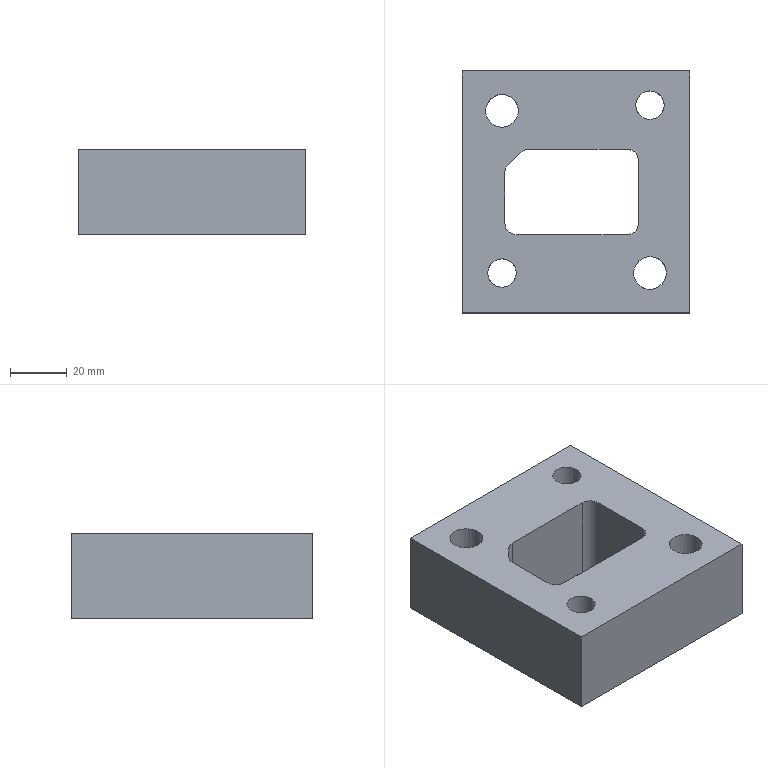Part | NX | features 7 2 | 1 solid | 28 faces | box 80 x 85 x 30 mm | volume 147731 mm3 | plane 15 | cylinder 13 | commonest cylinder face diameters 8 x5 10.001 x2 10.31 x2 11.5 x2 18 x2
STEP:
#1=CARTESIAN_POINT('',(3138.247,112.829,91.));
#2=VERTEX_POINT('',#1);
#3=CARTESIAN_POINT('',(3138.247,107.828,91.));
#4=DIRECTION('',(0.,0.,-1.));
#5=DIRECTION('',(0.,1.,0.));
#6=AXIS2_PLACEMENT_3D('',#3,#4,#5);
#7=CIRCLE('',#6,5.);
#8=EDGE_CURVE('',#2,#2,#7,.T.);
#9=ORIENTED_EDGE('',*,*,#8,.T.);
#10=EDGE_LOOP('',(#9));
#11=FACE_BOUND('',#10,.T.);
#12=CARTESIAN_POINT('',(3086.247,111.578,91.));
#13=VERTEX_POINT('',#12);
#14=CARTESIAN_POINT('',(3086.247,105.828,91.));
#15=DIRECTION('',(0.,0.,1.));
#16=DIRECTION('',(0.,1.,0.));
#17=AXIS2_PLACEMENT_3D('',#14,#15,#16);
#18=CIRCLE('',#17,5.75);
#19=EDGE_CURVE('',#13,#13,#18,.T.);
#20=ORIENTED_EDGE('',*,*,#19,.F.);
#21=EDGE_LOOP('',(#20));
#22=FACE_BOUND('',#21,.T.);
#23=CARTESIAN_POINT('',(3152.247,34.828,91.));
#24=VERTEX_POINT('',#23);
#25=CARTESIAN_POINT('',(3072.247,34.828,91.));
#26=VERTEX_POINT('',#25);
#27=CARTESIAN_POINT('',(3102.247,34.828,91.));
#28=DIRECTION('',(-1.,0.,0.));
#29=VECTOR('',#28,1000.);
#30=LINE('',#27,#29);
#31=EDGE_CURVE('',#24,#26,#30,.T.);
#32=ORIENTED_EDGE('',*,*,#31,.F.);
#33=CARTESIAN_POINT('',(3152.247,119.828,91.));
#34=VERTEX_POINT('',#33);
#35=CARTESIAN_POINT('',(3152.247,77.328,91.));
#36=DIRECTION('',(0.,-1.,0.));
#37=VECTOR('',#36,1000.);
#38=LINE('',#35,#37);
#39=EDGE_CURVE('',#34,#24,#38,.T.);
#40=ORIENTED_EDGE('',*,*,#39,.F.);
#41=CARTESIAN_POINT('',(3072.247,119.828,91.));
#42=VERTEX_POINT('',#41);
#43=CARTESIAN_POINT('',(3102.247,119.828,91.));
#44=DIRECTION('',(1.,0.,0.));
#45=VECTOR('',#44,1000.);
#46=LINE('',#43,#45);
#47=EDGE_CURVE('',#42,#34,#46,.T.);
#48=ORIENTED_EDGE('',*,*,#47,.F.);
#49=CARTESIAN_POINT('',(3072.247,77.328,91.));
#50=DIRECTION('',(0.,1.,0.));
#51=VECTOR('',#50,1000.);
#52=LINE('',#49,#51);
#53=EDGE_CURVE('',#26,#42,#52,.T.);
#54=ORIENTED_EDGE('',*,*,#53,.F.);
#55=EDGE_LOOP('',(#32,#40,#48,#54));
#56=FACE_BOUND('',#55,.T.);
#57=CARTESIAN_POINT('',(3138.247,54.578,91.));
#58=VERTEX_POINT('',#57);
#59=CARTESIAN_POINT('',(3138.247,48.828,91.));
#60=DIRECTION('',(0.,0.,1.));
#61=DIRECTION('',(0.,1.,0.));
#62=AXIS2_PLACEMENT_3D('',#59,#60,#61);
#63=CIRCLE('',#62,5.75);
#64=EDGE_CURVE('',#58,#58,#63,.T.);
#65=ORIENTED_EDGE('',*,*,#64,.F.);
#66=EDGE_LOOP('',(#65));
#67=FACE_BOUND('',#66,.T.);
#68=CARTESIAN_POINT('',(3086.247,53.829,91.));
#69=VERTEX_POINT('',#68);
#70=CARTESIAN_POINT('',(3086.247,48.828,91.));
#71=DIRECTION('',(0.,0.,-1.));
#72=DIRECTION('',(0.,1.,0.));
#73=AXIS2_PLACEMENT_3D('',#70,#71,#72);
#74=CIRCLE('',#73,5.);
#75=EDGE_CURVE('',#69,#69,#74,.T.);
#76=ORIENTED_EDGE('',*,*,#75,.T.);
#77=EDGE_LOOP('',(#76));
#78=FACE_BOUND('',#77,.T.);
#79=CARTESIAN_POINT('',(3130.247,62.328,91.));
#80=VERTEX_POINT('',#79);
#81=CARTESIAN_POINT('',(3134.247,66.328,91.));
#82=VERTEX_POINT('',#81);
#83=CARTESIAN_POINT('',(3130.247,66.328,91.));
#84=DIRECTION('',(0.,0.,1.));
#85=DIRECTION('',(0.,1.,0.));
#86=AXIS2_PLACEMENT_3D('',#83,#84,#85);
#87=CIRCLE('',#86,4.);
#88=EDGE_CURVE('',#80,#82,#87,.T.);
#89=ORIENTED_EDGE('',*,*,#88,.F.);
#90=CARTESIAN_POINT('',(3091.247,62.328,91.));
#91=VERTEX_POINT('',#90);
#92=CARTESIAN_POINT('',(3102.247,62.328,91.));
#93=DIRECTION('',(-1.,0.,0.));
#94=VECTOR('',#93,1000.);
#95=LINE('',#92,#94);
#96=EDGE_CURVE('',#80,#91,#95,.T.);
#97=ORIENTED_EDGE('',*,*,#96,.T.);
#98=CARTESIAN_POINT('',(3087.247,66.328,91.));
#99=VERTEX_POINT('',#98);
#100=CARTESIAN_POINT('',(3091.247,66.328,91.));
#101=DIRECTION('',(0.,0.,1.));
#102=DIRECTION('',(0.,1.,0.));
#103=AXIS2_PLACEMENT_3D('',#100,#101,#102);
#104=CIRCLE('',#103,4.);
#105=EDGE_CURVE('',#99,#91,#104,.T.);
#106=ORIENTED_EDGE('',*,*,#105,.F.);
#107=CARTESIAN_POINT('',(3087.247,84.035,91.));
#108=VERTEX_POINT('',#107);
#109=CARTESIAN_POINT('',(3087.247,77.328,91.));
#110=DIRECTION('',(0.,1.,0.));
#111=VECTOR('',#110,1000.);
#112=LINE('',#109,#111);
#113=EDGE_CURVE('',#99,#108,#112,.T.);
#114=ORIENTED_EDGE('',*,*,#113,.T.);
#115=CARTESIAN_POINT('',(3088.419,86.864,91.));
#116=VERTEX_POINT('',#115);
#117=CARTESIAN_POINT('',(3091.247,84.035,91.));
#118=DIRECTION('',(0.,0.,1.));
#119=DIRECTION('',(0.,1.,0.));
#120=AXIS2_PLACEMENT_3D('',#117,#118,#119);
#121=CIRCLE('',#120,4.);
#122=EDGE_CURVE('',#116,#108,#121,.T.);
#123=ORIENTED_EDGE('',*,*,#122,.F.);
#124=CARTESIAN_POINT('',(3092.711,91.157,91.));
#125=VERTEX_POINT('',#124);
#126=CARTESIAN_POINT('',(3091.815,90.26,91.));
#127=DIRECTION('',(-0.7071,-0.7071,0.));
#128=VECTOR('',#127,1000.);
#129=LINE('',#126,#128);
#130=EDGE_CURVE('',#125,#116,#129,.T.);
#131=ORIENTED_EDGE('',*,*,#130,.F.);
#132=CARTESIAN_POINT('',(3095.54,92.328,91.));
#133=VERTEX_POINT('',#132);
#134=CARTESIAN_POINT('',(3095.54,88.328,91.));
#135=DIRECTION('',(0.,0.,1.));
#136=DIRECTION('',(0.,1.,0.));
#137=AXIS2_PLACEMENT_3D('',#134,#135,#136);
#138=CIRCLE('',#137,4.);
#139=EDGE_CURVE('',#133,#125,#138,.T.);
#140=ORIENTED_EDGE('',*,*,#139,.F.);
#141=CARTESIAN_POINT('',(3130.247,92.328,91.));
#142=VERTEX_POINT('',#141);
#143=CARTESIAN_POINT('',(3102.247,92.328,91.));
#144=DIRECTION('',(1.,0.,0.));
#145=VECTOR('',#144,1000.);
#146=LINE('',#143,#145);
#147=EDGE_CURVE('',#133,#142,#146,.T.);
#148=ORIENTED_EDGE('',*,*,#147,.T.);
#149=CARTESIAN_POINT('',(3134.247,88.328,91.));
#150=VERTEX_POINT('',#149);
#151=CARTESIAN_POINT('',(3130.247,88.328,91.));
#152=DIRECTION('',(0.,0.,1.));
#153=DIRECTION('',(0.,1.,0.));
#154=AXIS2_PLACEMENT_3D('',#151,#152,#153);
#155=CIRCLE('',#154,4.);
#156=EDGE_CURVE('',#150,#142,#155,.T.);
#157=ORIENTED_EDGE('',*,*,#156,.F.);
#158=CARTESIAN_POINT('',(3134.247,77.328,91.));
#159=DIRECTION('',(0.,-1.,0.));
#160=VECTOR('',#159,1000.);
#161=LINE('',#158,#160);
#162=EDGE_CURVE('',#150,#82,#161,.T.);
#163=ORIENTED_EDGE('',*,*,#162,.T.);
#164=EDGE_LOOP('',(#89,#97,#106,#114,#123,#131,#140,#148,#157,#163));
#165=FACE_BOUND('',#164,.T.);
#166=CARTESIAN_POINT('',(3102.247,77.328,91.));
#167=DIRECTION('',(0.,0.,1.));
#168=DIRECTION('',(0.,-1.,0.));
#169=AXIS2_PLACEMENT_3D('',#166,#167,#168);
#170=PLANE('',#169);
#171=ADVANCED_FACE('',(#11,#22,#56,#67,#78,#165),#170,.T.);
#172=CARTESIAN_POINT('',(3143.402,107.828,61.));
#173=VERTEX_POINT('',#172);
#174=CARTESIAN_POINT('',(3138.247,107.828,61.));
#175=DIRECTION('',(0.,0.,1.));
#176=DIRECTION('',(1.,0.,0.));
#177=AXIS2_PLACEMENT_3D('',#174,#175,#176);
#178=CIRCLE('',#177,5.155);
#179=EDGE_CURVE('',#173,#173,#178,.T.);
#180=ORIENTED_EDGE('',*,*,#179,.T.);
#181=EDGE_LOOP('',(#180));
#182=FACE_BOUND('',#181,.T.);
#183=CARTESIAN_POINT('',(3091.402,48.828,61.));
#184=VERTEX_POINT('',#183);
#185=CARTESIAN_POINT('',(3086.247,48.828,61.));
#186=DIRECTION('',(0.,0.,1.));
#187=DIRECTION('',(1.,0.,0.));
#188=AXIS2_PLACEMENT_3D('',#185,#186,#187);
#189=CIRCLE('',#188,5.155);
#190=EDGE_CURVE('',#184,#184,#189,.T.);
#191=ORIENTED_EDGE('',*,*,#190,.T.);
#192=EDGE_LOOP('',(#191));
#193=FACE_BOUND('',#192,.T.);
#194=CARTESIAN_POINT('',(3072.247,119.828,61.));
#195=VERTEX_POINT('',#194);
#196=CARTESIAN_POINT('',(3072.247,34.828,61.));
#197=VERTEX_POINT('',#196);
#198=CARTESIAN_POINT('',(3072.247,-99.672,61.));
#199=DIRECTION('',(0.,-1.,0.));
#200=VECTOR('',#199,1000.);
#201=LINE('',#198,#200);
#202=EDGE_CURVE('',#195,#197,#201,.T.);
#203=ORIENTED_EDGE('',*,*,#202,.F.);
#204=CARTESIAN_POINT('',(3152.247,119.828,61.));
#205=VERTEX_POINT('',#204);
#206=CARTESIAN_POINT('',(3287.247,119.828,61.));
#207=DIRECTION('',(-1.,0.,0.));
#208=VECTOR('',#207,1000.);
#209=LINE('',#206,#208);
#210=EDGE_CURVE('',#205,#195,#209,.T.);
#211=ORIENTED_EDGE('',*,*,#210,.F.);
#212=CARTESIAN_POINT('',(3152.247,34.828,61.));
#213=VERTEX_POINT('',#212);
#214=CARTESIAN_POINT('',(3152.247,-99.672,61.));
#215=DIRECTION('',(0.,1.,0.));
#216=VECTOR('',#215,1000.);
#217=LINE('',#214,#216);
#218=EDGE_CURVE('',#213,#205,#217,.T.);
#219=ORIENTED_EDGE('',*,*,#218,.F.);
#220=CARTESIAN_POINT('',(3287.247,34.828,61.));
#221=DIRECTION('',(1.,0.,0.));
#222=VECTOR('',#221,1000.);
#223=LINE('',#220,#222);
#224=EDGE_CURVE('',#197,#213,#223,.T.);
#225=ORIENTED_EDGE('',*,*,#224,.F.);
#226=EDGE_LOOP('',(#203,#211,#219,#225));
#227=FACE_BOUND('',#226,.T.);
#228=CARTESIAN_POINT('',(3129.247,48.828,61.));
#229=VERTEX_POINT('',#228);
#230=CARTESIAN_POINT('',(3138.247,48.828,61.));
#231=DIRECTION('',(0.,0.,1.));
#232=DIRECTION('',(-1.,0.,0.));
#233=AXIS2_PLACEMENT_3D('',#230,#231,#232);
#234=CIRCLE('',#233,9.);
#235=EDGE_CURVE('',#229,#229,#234,.T.);
#236=ORIENTED_EDGE('',*,*,#235,.T.);
#237=EDGE_LOOP('',(#236));
#238=FACE_BOUND('',#237,.T.);
#239=CARTESIAN_POINT('',(3077.247,105.828,61.));
#240=VERTEX_POINT('',#239);
#241=CARTESIAN_POINT('',(3086.247,105.828,61.));
#242=DIRECTION('',(0.,0.,1.));
#243=DIRECTION('',(-1.,0.,0.));
#244=AXIS2_PLACEMENT_3D('',#241,#242,#243);
#245=CIRCLE('',#244,9.);
#246=EDGE_CURVE('',#240,#240,#245,.T.);
#247=ORIENTED_EDGE('',*,*,#246,.T.);
#248=EDGE_LOOP('',(#247));
#249=FACE_BOUND('',#248,.T.);
#250=CARTESIAN_POINT('',(3134.247,66.328,61.));
#251=VERTEX_POINT('',#250);
#252=CARTESIAN_POINT('',(3130.247,62.328,61.));
#253=VERTEX_POINT('',#252);
#254=CARTESIAN_POINT('',(3130.247,66.328,61.));
#255=DIRECTION('',(0.,0.,-1.));
#256=DIRECTION('',(-1.,0.,0.));
#257=AXIS2_PLACEMENT_3D('',#254,#255,#256);
#258=CIRCLE('',#257,4.);
#259=EDGE_CURVE('',#251,#253,#258,.T.);
#260=ORIENTED_EDGE('',*,*,#259,.F.);
#261=CARTESIAN_POINT('',(3134.247,88.328,61.));
#262=VERTEX_POINT('',#261);
#263=CARTESIAN_POINT('',(3134.247,-99.672,61.));
#264=DIRECTION('',(0.,1.,0.));
#265=VECTOR('',#264,1000.);
#266=LINE('',#263,#265);
#267=EDGE_CURVE('',#251,#262,#266,.T.);
#268=ORIENTED_EDGE('',*,*,#267,.T.);
#269=CARTESIAN_POINT('',(3130.247,92.328,61.));
#270=VERTEX_POINT('',#269);
#271=CARTESIAN_POINT('',(3130.247,88.328,61.));
#272=DIRECTION('',(0.,0.,-1.));
#273=DIRECTION('',(-1.,0.,0.));
#274=AXIS2_PLACEMENT_3D('',#271,#272,#273);
#275=CIRCLE('',#274,4.);
#276=EDGE_CURVE('',#270,#262,#275,.T.);
#277=ORIENTED_EDGE('',*,*,#276,.F.);
#278=CARTESIAN_POINT('',(3095.54,92.328,61.));
#279=VERTEX_POINT('',#278);
#280=CARTESIAN_POINT('',(3287.247,92.328,61.));
#281=DIRECTION('',(-1.,0.,0.));
#282=VECTOR('',#281,1000.);
#283=LINE('',#280,#282);
#284=EDGE_CURVE('',#270,#279,#283,.T.);
#285=ORIENTED_EDGE('',*,*,#284,.T.);
#286=CARTESIAN_POINT('',(3092.711,91.157,61.));
#287=VERTEX_POINT('',#286);
#288=CARTESIAN_POINT('',(3095.54,88.328,61.));
#289=DIRECTION('',(0.,0.,-1.));
#290=DIRECTION('',(-1.,0.,0.));
#291=AXIS2_PLACEMENT_3D('',#288,#289,#290);
#292=CIRCLE('',#291,4.);
#293=EDGE_CURVE('',#287,#279,#292,.T.);
#294=ORIENTED_EDGE('',*,*,#293,.F.);
#295=CARTESIAN_POINT('',(3088.419,86.864,61.));
#296=VERTEX_POINT('',#295);
#297=CARTESIAN_POINT('',(3094.565,93.01,61.));
#298=DIRECTION('',(0.7071,0.7071,0.));
#299=VECTOR('',#298,1000.);
#300=LINE('',#297,#299);
#301=EDGE_CURVE('',#296,#287,#300,.T.);
#302=ORIENTED_EDGE('',*,*,#301,.F.);
#303=CARTESIAN_POINT('',(3087.247,84.035,61.));
#304=VERTEX_POINT('',#303);
#305=CARTESIAN_POINT('',(3091.247,84.035,61.));
#306=DIRECTION('',(0.,0.,-1.));
#307=DIRECTION('',(-1.,0.,0.));
#308=AXIS2_PLACEMENT_3D('',#305,#306,#307);
#309=CIRCLE('',#308,4.);
#310=EDGE_CURVE('',#304,#296,#309,.T.);
#311=ORIENTED_EDGE('',*,*,#310,.F.);
#312=CARTESIAN_POINT('',(3087.247,66.328,61.));
#313=VERTEX_POINT('',#312);
#314=CARTESIAN_POINT('',(3087.247,-99.672,61.));
#315=DIRECTION('',(0.,-1.,0.));
#316=VECTOR('',#315,1000.);
#317=LINE('',#314,#316);
#318=EDGE_CURVE('',#304,#313,#317,.T.);
#319=ORIENTED_EDGE('',*,*,#318,.T.);
#320=CARTESIAN_POINT('',(3091.247,62.328,61.));
#321=VERTEX_POINT('',#320);
#322=CARTESIAN_POINT('',(3091.247,66.328,61.));
#323=DIRECTION('',(0.,0.,-1.));
#324=DIRECTION('',(-1.,0.,0.));
#325=AXIS2_PLACEMENT_3D('',#322,#323,#324);
#326=CIRCLE('',#325,4.);
#327=EDGE_CURVE('',#321,#313,#326,.T.);
#328=ORIENTED_EDGE('',*,*,#327,.F.);
#329=CARTESIAN_POINT('',(3287.247,62.328,61.));
#330=DIRECTION('',(1.,0.,0.));
#331=VECTOR('',#330,1000.);
#332=LINE('',#329,#331);
#333=EDGE_CURVE('',#321,#253,#332,.T.);
#334=ORIENTED_EDGE('',*,*,#333,.T.);
#335=EDGE_LOOP('',(#260,#268,#277,#285,#294,#302,#311,#319,#328,#334));
#336=FACE_BOUND('',#335,.T.);
#337=CARTESIAN_POINT('',(3287.247,-99.672,61.));
#338=DIRECTION('',(0.,0.,-1.));
#339=DIRECTION('',(0.,1.,0.));
#340=AXIS2_PLACEMENT_3D('',#337,#338,#339);
#341=PLANE('',#340);
#342=ADVANCED_FACE('',(#182,#193,#227,#238,#249,#336),#341,.T.);
#343=ORIENTED_EDGE('',*,*,#53,.T.);
#344=CARTESIAN_POINT('',(3072.247,119.828,6.933));
#345=DIRECTION('',(0.,0.,-1.));
#346=VECTOR('',#345,1000.);
#347=LINE('',#344,#346);
#348=EDGE_CURVE('',#42,#195,#347,.T.);
#349=ORIENTED_EDGE('',*,*,#348,.T.);
#350=ORIENTED_EDGE('',*,*,#202,.T.);
#351=CARTESIAN_POINT('',(3072.247,34.828,6.933));
#352=DIRECTION('',(0.,0.,-1.));
#353=VECTOR('',#352,1000.);
#354=LINE('',#351,#353);
#355=EDGE_CURVE('',#26,#197,#354,.T.);
#356=ORIENTED_EDGE('',*,*,#355,.F.);
#357=EDGE_LOOP('',(#343,#349,#350,#356));
#358=FACE_BOUND('',#357,.T.);
#359=CARTESIAN_POINT('',(3072.247,77.328,6.933));
#360=DIRECTION('',(-1.,0.,0.));
#361=DIRECTION('',(0.,0.,-1.));
#362=AXIS2_PLACEMENT_3D('',#359,#360,#361);
#363=PLANE('',#362);
#364=ADVANCED_FACE('',(#358),#363,.T.);
#365=ORIENTED_EDGE('',*,*,#47,.T.);
#366=CARTESIAN_POINT('',(3152.247,119.828,6.933));
#367=DIRECTION('',(0.,0.,-1.));
#368=VECTOR('',#367,1000.);
#369=LINE('',#366,#368);
#370=EDGE_CURVE('',#34,#205,#369,.T.);
#371=ORIENTED_EDGE('',*,*,#370,.T.);
#372=ORIENTED_EDGE('',*,*,#210,.T.);
#373=ORIENTED_EDGE('',*,*,#348,.F.);
#374=EDGE_LOOP('',(#365,#371,#372,#373));
#375=FACE_BOUND('',#374,.T.);
#376=CARTESIAN_POINT('',(3102.247,119.828,6.933));
#377=DIRECTION('',(0.,1.,0.));
#378=DIRECTION('',(0.,0.,1.));
#379=AXIS2_PLACEMENT_3D('',#376,#377,#378);
#380=PLANE('',#379);
#381=ADVANCED_FACE('',(#375),#380,.T.);
#382=ORIENTED_EDGE('',*,*,#39,.T.);
#383=CARTESIAN_POINT('',(3152.247,34.828,6.933));
#384=DIRECTION('',(0.,0.,1.));
#385=VECTOR('',#384,1000.);
#386=LINE('',#383,#385);
#387=EDGE_CURVE('',#213,#24,#386,.T.);
#388=ORIENTED_EDGE('',*,*,#387,.F.);
#389=ORIENTED_EDGE('',*,*,#218,.T.);
#390=ORIENTED_EDGE('',*,*,#370,.F.);
#391=EDGE_LOOP('',(#382,#388,#389,#390));
#392=FACE_BOUND('',#391,.T.);
#393=CARTESIAN_POINT('',(3152.247,77.328,6.933));
#394=DIRECTION('',(1.,0.,0.));
#395=DIRECTION('',(0.,0.,1.));
#396=AXIS2_PLACEMENT_3D('',#393,#394,#395);
#397=PLANE('',#396);
#398=ADVANCED_FACE('',(#392),#397,.T.);
#399=ORIENTED_EDGE('',*,*,#224,.T.);
#400=ORIENTED_EDGE('',*,*,#387,.T.);
#401=ORIENTED_EDGE('',*,*,#31,.T.);
#402=ORIENTED_EDGE('',*,*,#355,.T.);
#403=EDGE_LOOP('',(#399,#400,#401,#402));
#404=FACE_BOUND('',#403,.T.);
#405=CARTESIAN_POINT('',(3102.247,34.828,6.933));
#406=DIRECTION('',(0.,-1.,0.));
#407=DIRECTION('',(0.,0.,-1.));
#408=AXIS2_PLACEMENT_3D('',#405,#406,#407);
#409=PLANE('',#408);
#410=ADVANCED_FACE('',(#404),#409,.T.);
#411=ORIENTED_EDGE('',*,*,#64,.T.);
#412=EDGE_LOOP('',(#411));
#413=FACE_BOUND('',#412,.T.);
#414=CARTESIAN_POINT('',(3143.997,48.828,74.));
#415=VERTEX_POINT('',#414);
#416=CARTESIAN_POINT('',(3138.247,48.828,74.));
#417=DIRECTION('',(0.,0.,1.));
#418=DIRECTION('',(1.,0.,0.));
#419=AXIS2_PLACEMENT_3D('',#416,#417,#418);
#420=CIRCLE('',#419,5.75);
#421=EDGE_CURVE('',#415,#415,#420,.T.);
#422=ORIENTED_EDGE('',*,*,#421,.F.);
#423=EDGE_LOOP('',(#422));
#424=FACE_BOUND('',#423,.T.);
#425=CARTESIAN_POINT('',(3138.247,48.828,51.));
#426=DIRECTION('',(0.,0.,1.));
#427=DIRECTION('',(0.,-1.,0.));
#428=AXIS2_PLACEMENT_3D('',#425,#426,#427);
#429=CYLINDRICAL_SURFACE('',#428,5.75);
#430=ADVANCED_FACE('',(#413,#424),#429,.F.);
#431=ORIENTED_EDGE('',*,*,#421,.T.);
#432=EDGE_LOOP('',(#431));
#433=FACE_BOUND('',#432,.T.);
#434=CARTESIAN_POINT('',(3147.247,48.828,74.));
#435=VERTEX_POINT('',#434);
#436=CARTESIAN_POINT('',(3138.247,48.828,74.));
#437=DIRECTION('',(0.,0.,1.));
#438=DIRECTION('',(1.,0.,0.));
#439=AXIS2_PLACEMENT_3D('',#436,#437,#438);
#440=CIRCLE('',#439,9.);
#441=EDGE_CURVE('',#435,#435,#440,.T.);
#442=ORIENTED_EDGE('',*,*,#441,.F.);
#443=EDGE_LOOP('',(#442));
#444=FACE_BOUND('',#443,.T.);
#445=CARTESIAN_POINT('',(3138.247,48.828,74.));
#446=DIRECTION('',(0.,0.,1.));
#447=DIRECTION('',(0.,-1.,0.));
#448=AXIS2_PLACEMENT_3D('',#445,#446,#447);
#449=PLANE('',#448);
#450=ADVANCED_FACE('',(#433,#444),#449,.F.);
#451=ORIENTED_EDGE('',*,*,#441,.T.);
#452=EDGE_LOOP('',(#451));
#453=FACE_BOUND('',#452,.T.);
#454=ORIENTED_EDGE('',*,*,#235,.F.);
#455=EDGE_LOOP('',(#454));
#456=FACE_BOUND('',#455,.T.);
#457=CARTESIAN_POINT('',(3138.247,48.828,56.));
#458=DIRECTION('',(0.,0.,1.));
#459=DIRECTION('',(0.,-1.,0.));
#460=AXIS2_PLACEMENT_3D('',#457,#458,#459);
#461=CYLINDRICAL_SURFACE('',#460,9.);
#462=ADVANCED_FACE('',(#453,#456),#461,.F.);
#463=CARTESIAN_POINT('',(3091.247,48.828,71.));
#464=VERTEX_POINT('',#463);
#465=CARTESIAN_POINT('',(3086.247,48.828,71.));
#466=DIRECTION('',(0.,0.,-1.));
#467=DIRECTION('',(1.,0.,0.));
#468=AXIS2_PLACEMENT_3D('',#465,#466,#467);
#469=CIRCLE('',#468,5.);
#470=EDGE_CURVE('',#464,#464,#469,.T.);
#471=ORIENTED_EDGE('',*,*,#470,.T.);
#472=EDGE_LOOP('',(#471));
#473=FACE_BOUND('',#472,.T.);
#474=ORIENTED_EDGE('',*,*,#75,.F.);
#475=EDGE_LOOP('',(#474));
#476=FACE_BOUND('',#475,.T.);
#477=CARTESIAN_POINT('',(3086.247,48.828,621.));
#478=DIRECTION('',(0.,0.,-1.));
#479=DIRECTION('',(0.,1.,0.));
#480=AXIS2_PLACEMENT_3D('',#477,#478,#479);
#481=CYLINDRICAL_SURFACE('',#480,5.);
#482=ADVANCED_FACE('',(#473,#476),#481,.F.);
#483=ORIENTED_EDGE('',*,*,#19,.T.);
#484=EDGE_LOOP('',(#483));
#485=FACE_BOUND('',#484,.T.);
#486=CARTESIAN_POINT('',(3091.997,105.828,74.));
#487=VERTEX_POINT('',#486);
#488=CARTESIAN_POINT('',(3086.247,105.828,74.));
#489=DIRECTION('',(0.,0.,1.));
#490=DIRECTION('',(1.,0.,0.));
#491=AXIS2_PLACEMENT_3D('',#488,#489,#490);
#492=CIRCLE('',#491,5.75);
#493=EDGE_CURVE('',#487,#487,#492,.T.);
#494=ORIENTED_EDGE('',*,*,#493,.F.);
#495=EDGE_LOOP('',(#494));
#496=FACE_BOUND('',#495,.T.);
#497=CARTESIAN_POINT('',(3086.247,105.828,51.));
#498=DIRECTION('',(0.,0.,1.));
#499=DIRECTION('',(0.,-1.,0.));
#500=AXIS2_PLACEMENT_3D('',#497,#498,#499);
#501=CYLINDRICAL_SURFACE('',#500,5.75);
#502=ADVANCED_FACE('',(#485,#496),#501,.F.);
#503=ORIENTED_EDGE('',*,*,#493,.T.);
#504=EDGE_LOOP('',(#503));
#505=FACE_BOUND('',#504,.T.);
#506=CARTESIAN_POINT('',(3095.247,105.828,74.));
#507=VERTEX_POINT('',#506);
#508=CARTESIAN_POINT('',(3086.247,105.828,74.));
#509=DIRECTION('',(0.,0.,1.));
#510=DIRECTION('',(1.,0.,0.));
#511=AXIS2_PLACEMENT_3D('',#508,#509,#510);
#512=CIRCLE('',#511,9.);
#513=EDGE_CURVE('',#507,#507,#512,.T.);
#514=ORIENTED_EDGE('',*,*,#513,.F.);
#515=EDGE_LOOP('',(#514));
#516=FACE_BOUND('',#515,.T.);
#517=CARTESIAN_POINT('',(3086.247,105.828,74.));
#518=DIRECTION('',(0.,0.,1.));
#519=DIRECTION('',(0.,-1.,0.));
#520=AXIS2_PLACEMENT_3D('',#517,#518,#519);
#521=PLANE('',#520);
#522=ADVANCED_FACE('',(#505,#516),#521,.F.);
#523=ORIENTED_EDGE('',*,*,#513,.T.);
#524=EDGE_LOOP('',(#523));
#525=FACE_BOUND('',#524,.T.);
#526=ORIENTED_EDGE('',*,*,#246,.F.);
#527=EDGE_LOOP('',(#526));
#528=FACE_BOUND('',#527,.T.);
#529=CARTESIAN_POINT('',(3086.247,105.828,56.));
#530=DIRECTION('',(0.,0.,1.));
#531=DIRECTION('',(0.,-1.,0.));
#532=AXIS2_PLACEMENT_3D('',#529,#530,#531);
#533=CYLINDRICAL_SURFACE('',#532,9.);
#534=ADVANCED_FACE('',(#525,#528),#533,.F.);
#535=CARTESIAN_POINT('',(3143.247,107.828,71.));
#536=VERTEX_POINT('',#535);
#537=CARTESIAN_POINT('',(3138.247,107.828,71.));
#538=DIRECTION('',(0.,0.,-1.));
#539=DIRECTION('',(1.,0.,0.));
#540=AXIS2_PLACEMENT_3D('',#537,#538,#539);
#541=CIRCLE('',#540,5.);
#542=EDGE_CURVE('',#536,#536,#541,.T.);
#543=ORIENTED_EDGE('',*,*,#542,.T.);
#544=EDGE_LOOP('',(#543));
#545=FACE_BOUND('',#544,.T.);
#546=ORIENTED_EDGE('',*,*,#8,.F.);
#547=EDGE_LOOP('',(#546));
#548=FACE_BOUND('',#547,.T.);
#549=CARTESIAN_POINT('',(3138.247,107.828,621.));
#550=DIRECTION('',(0.,0.,-1.));
#551=DIRECTION('',(0.,1.,0.));
#552=AXIS2_PLACEMENT_3D('',#549,#550,#551);
#553=CYLINDRICAL_SURFACE('',#552,5.);
#554=ADVANCED_FACE('',(#545,#548),#553,.F.);
#555=ORIENTED_EDGE('',*,*,#113,.F.);
#556=CARTESIAN_POINT('',(3087.247,66.328,-5.));
#557=DIRECTION('',(0.,0.,-1.));
#558=VECTOR('',#557,1000.);
#559=LINE('',#556,#558);
#560=EDGE_CURVE('',#99,#313,#559,.T.);
#561=ORIENTED_EDGE('',*,*,#560,.T.);
#562=ORIENTED_EDGE('',*,*,#318,.F.);
#563=CARTESIAN_POINT('',(3087.247,84.035,-5.));
#564=DIRECTION('',(0.,0.,1.));
#565=VECTOR('',#564,1000.);
#566=LINE('',#563,#565);
#567=EDGE_CURVE('',#304,#108,#566,.T.);
#568=ORIENTED_EDGE('',*,*,#567,.T.);
#569=EDGE_LOOP('',(#555,#561,#562,#568));
#570=FACE_BOUND('',#569,.T.);
#571=CARTESIAN_POINT('',(3087.247,77.328,-5.));
#572=DIRECTION('',(-1.,0.,0.));
#573=DIRECTION('',(0.,0.,-1.));
#574=AXIS2_PLACEMENT_3D('',#571,#572,#573);
#575=PLANE('',#574);
#576=ADVANCED_FACE('',(#570),#575,.F.);
#577=ORIENTED_EDGE('',*,*,#147,.F.);
#578=CARTESIAN_POINT('',(3095.54,92.328,-5.));
#579=DIRECTION('',(0.,0.,-1.));
#580=VECTOR('',#579,1000.);
#581=LINE('',#578,#580);
#582=EDGE_CURVE('',#133,#279,#581,.T.);
#583=ORIENTED_EDGE('',*,*,#582,.T.);
#584=ORIENTED_EDGE('',*,*,#284,.F.);
#585=CARTESIAN_POINT('',(3130.247,92.328,-5.));
#586=DIRECTION('',(0.,0.,1.));
#587=VECTOR('',#586,1000.);
#588=LINE('',#585,#587);
#589=EDGE_CURVE('',#270,#142,#588,.T.);
#590=ORIENTED_EDGE('',*,*,#589,.T.);
#591=EDGE_LOOP('',(#577,#583,#584,#590));
#592=FACE_BOUND('',#591,.T.);
#593=CARTESIAN_POINT('',(3102.247,92.328,-5.));
#594=DIRECTION('',(0.,1.,0.));
#595=DIRECTION('',(0.,0.,1.));
#596=AXIS2_PLACEMENT_3D('',#593,#594,#595);
#597=PLANE('',#596);
#598=ADVANCED_FACE('',(#592),#597,.F.);
#599=ORIENTED_EDGE('',*,*,#162,.F.);
#600=CARTESIAN_POINT('',(3134.247,88.328,-5.));
#601=DIRECTION('',(0.,0.,-1.));
#602=VECTOR('',#601,1000.);
#603=LINE('',#600,#602);
#604=EDGE_CURVE('',#150,#262,#603,.T.);
#605=ORIENTED_EDGE('',*,*,#604,.T.);
#606=ORIENTED_EDGE('',*,*,#267,.F.);
#607=CARTESIAN_POINT('',(3134.247,66.328,-5.));
#608=DIRECTION('',(0.,0.,1.));
#609=VECTOR('',#608,1000.);
#610=LINE('',#607,#609);
#611=EDGE_CURVE('',#251,#82,#610,.T.);
#612=ORIENTED_EDGE('',*,*,#611,.T.);
#613=EDGE_LOOP('',(#599,#605,#606,#612));
#614=FACE_BOUND('',#613,.T.);
#615=CARTESIAN_POINT('',(3134.247,77.328,-5.));
#616=DIRECTION('',(1.,0.,0.));
#617=DIRECTION('',(0.,0.,1.));
#618=AXIS2_PLACEMENT_3D('',#615,#616,#617);
#619=PLANE('',#618);
#620=ADVANCED_FACE('',(#614),#619,.F.);
#621=ORIENTED_EDGE('',*,*,#333,.F.);
#622=CARTESIAN_POINT('',(3091.247,62.328,-5.));
#623=DIRECTION('',(0.,0.,1.));
#624=VECTOR('',#623,1000.);
#625=LINE('',#622,#624);
#626=EDGE_CURVE('',#321,#91,#625,.T.);
#627=ORIENTED_EDGE('',*,*,#626,.T.);
#628=ORIENTED_EDGE('',*,*,#96,.F.);
#629=CARTESIAN_POINT('',(3130.247,62.328,-5.));
#630=DIRECTION('',(0.,0.,-1.));
#631=VECTOR('',#630,1000.);
#632=LINE('',#629,#631);
#633=EDGE_CURVE('',#80,#253,#632,.T.);
#634=ORIENTED_EDGE('',*,*,#633,.T.);
#635=EDGE_LOOP('',(#621,#627,#628,#634));
#636=FACE_BOUND('',#635,.T.);
#637=CARTESIAN_POINT('',(3102.247,62.328,-5.));
#638=DIRECTION('',(0.,-1.,0.));
#639=DIRECTION('',(0.,0.,-1.));
#640=AXIS2_PLACEMENT_3D('',#637,#638,#639);
#641=PLANE('',#640);
#642=ADVANCED_FACE('',(#636),#641,.F.);
#643=ORIENTED_EDGE('',*,*,#130,.T.);
#644=CARTESIAN_POINT('',(3088.419,86.864,-5.));
#645=DIRECTION('',(0.,0.,-1.));
#646=VECTOR('',#645,1000.);
#647=LINE('',#644,#646);
#648=EDGE_CURVE('',#116,#296,#647,.T.);
#649=ORIENTED_EDGE('',*,*,#648,.T.);
#650=ORIENTED_EDGE('',*,*,#301,.T.);
#651=CARTESIAN_POINT('',(3092.711,91.157,-5.));
#652=DIRECTION('',(0.,0.,1.));
#653=VECTOR('',#652,1000.);
#654=LINE('',#651,#653);
#655=EDGE_CURVE('',#287,#125,#654,.T.);
#656=ORIENTED_EDGE('',*,*,#655,.T.);
#657=EDGE_LOOP('',(#643,#649,#650,#656));
#658=FACE_BOUND('',#657,.T.);
#659=CARTESIAN_POINT('',(3094.565,93.01,-5.));
#660=DIRECTION('',(0.7071,-0.7071,0.));
#661=DIRECTION('',(0.,0.,1.));
#662=AXIS2_PLACEMENT_3D('',#659,#660,#661);
#663=PLANE('',#662);
#664=ADVANCED_FACE('',(#658),#663,.T.);
#665=ORIENTED_EDGE('',*,*,#259,.T.);
#666=ORIENTED_EDGE('',*,*,#633,.F.);
#667=ORIENTED_EDGE('',*,*,#88,.T.);
#668=ORIENTED_EDGE('',*,*,#611,.F.);
#669=EDGE_LOOP('',(#665,#666,#667,#668));
#670=FACE_BOUND('',#669,.T.);
#671=CARTESIAN_POINT('',(3130.247,66.328,-5.));
#672=DIRECTION('',(0.,0.,-1.));
#673=DIRECTION('',(0.,-1.,0.));
#674=AXIS2_PLACEMENT_3D('',#671,#672,#673);
#675=CYLINDRICAL_SURFACE('',#674,4.);
#676=ADVANCED_FACE('',(#670),#675,.F.);
#677=ORIENTED_EDGE('',*,*,#276,.T.);
#678=ORIENTED_EDGE('',*,*,#604,.F.);
#679=ORIENTED_EDGE('',*,*,#156,.T.);
#680=ORIENTED_EDGE('',*,*,#589,.F.);
#681=EDGE_LOOP('',(#677,#678,#679,#680));
#682=FACE_BOUND('',#681,.T.);
#683=CARTESIAN_POINT('',(3130.247,88.328,-5.));
#684=DIRECTION('',(0.,0.,-1.));
#685=DIRECTION('',(0.,-1.,0.));
#686=AXIS2_PLACEMENT_3D('',#683,#684,#685);
#687=CYLINDRICAL_SURFACE('',#686,4.);
#688=ADVANCED_FACE('',(#682),#687,.F.);
#689=ORIENTED_EDGE('',*,*,#293,.T.);
#690=ORIENTED_EDGE('',*,*,#582,.F.);
#691=ORIENTED_EDGE('',*,*,#139,.T.);
#692=ORIENTED_EDGE('',*,*,#655,.F.);
#693=EDGE_LOOP('',(#689,#690,#691,#692));
#694=FACE_BOUND('',#693,.T.);
#695=CARTESIAN_POINT('',(3095.54,88.328,-5.));
#696=DIRECTION('',(0.,0.,1.));
#697=DIRECTION('',(0.,1.,0.));
#698=AXIS2_PLACEMENT_3D('',#695,#696,#697);
#699=CYLINDRICAL_SURFACE('',#698,4.);
#700=ADVANCED_FACE('',(#694),#699,.F.);
#701=ORIENTED_EDGE('',*,*,#122,.T.);
#702=ORIENTED_EDGE('',*,*,#567,.F.);
#703=ORIENTED_EDGE('',*,*,#310,.T.);
#704=ORIENTED_EDGE('',*,*,#648,.F.);
#705=EDGE_LOOP('',(#701,#702,#703,#704));
#706=FACE_BOUND('',#705,.T.);
#707=CARTESIAN_POINT('',(3091.247,84.035,-5.));
#708=DIRECTION('',(0.,0.,-1.));
#709=DIRECTION('',(0.,-1.,0.));
#710=AXIS2_PLACEMENT_3D('',#707,#708,#709);
#711=CYLINDRICAL_SURFACE('',#710,4.);
#712=ADVANCED_FACE('',(#706),#711,.F.);
#713=ORIENTED_EDGE('',*,*,#327,.T.);
#714=ORIENTED_EDGE('',*,*,#560,.F.);
#715=ORIENTED_EDGE('',*,*,#105,.T.);
#716=ORIENTED_EDGE('',*,*,#626,.F.);
#717=EDGE_LOOP('',(#713,#714,#715,#716));
#718=FACE_BOUND('',#717,.T.);
#719=CARTESIAN_POINT('',(3091.247,66.328,-5.));
#720=DIRECTION('',(0.,0.,-1.));
#721=DIRECTION('',(0.,-1.,0.));
#722=AXIS2_PLACEMENT_3D('',#719,#720,#721);
#723=CYLINDRICAL_SURFACE('',#722,4.);
#724=ADVANCED_FACE('',(#718),#723,.F.);
#725=CARTESIAN_POINT('',(3091.402,48.828,71.));
#726=VERTEX_POINT('',#725);
#727=CARTESIAN_POINT('',(3086.247,48.828,71.));
#728=DIRECTION('',(0.,0.,-1.));
#729=DIRECTION('',(1.,0.,0.));
#730=AXIS2_PLACEMENT_3D('',#727,#728,#729);
#731=CIRCLE('',#730,5.155);
#732=EDGE_CURVE('',#726,#726,#731,.T.);
#733=ORIENTED_EDGE('',*,*,#732,.T.);
#734=EDGE_LOOP('',(#733));
#735=FACE_BOUND('',#734,.T.);
#736=ORIENTED_EDGE('',*,*,#470,.F.);
#737=EDGE_LOOP('',(#736));
#738=FACE_BOUND('',#737,.T.);
#739=CARTESIAN_POINT('',(3086.247,48.828,71.));
#740=DIRECTION('',(0.,0.,1.));
#741=DIRECTION('',(-1.,0.,0.));
#742=AXIS2_PLACEMENT_3D('',#739,#740,#741);
#743=PLANE('',#742);
#744=ADVANCED_FACE('',(#735,#738),#743,.F.);
#745=ORIENTED_EDGE('',*,*,#732,.F.);
#746=EDGE_LOOP('',(#745));
#747=FACE_BOUND('',#746,.T.);
#748=ORIENTED_EDGE('',*,*,#190,.F.);
#749=EDGE_LOOP('',(#748));
#750=FACE_BOUND('',#749,.T.);
#751=CARTESIAN_POINT('',(3086.247,48.828,61.));
#752=DIRECTION('',(0.,0.,1.));
#753=DIRECTION('',(-1.,0.,0.));
#754=AXIS2_PLACEMENT_3D('',#751,#752,#753);
#755=CYLINDRICAL_SURFACE('',#754,5.155);
#756=ADVANCED_FACE('',(#747,#750),#755,.F.);
#757=CARTESIAN_POINT('',(3143.402,107.828,71.));
#758=VERTEX_POINT('',#757);
#759=CARTESIAN_POINT('',(3138.247,107.828,71.));
#760=DIRECTION('',(0.,0.,-1.));
#761=DIRECTION('',(1.,0.,0.));
#762=AXIS2_PLACEMENT_3D('',#759,#760,#761);
#763=CIRCLE('',#762,5.155);
#764=EDGE_CURVE('',#758,#758,#763,.T.);
#765=ORIENTED_EDGE('',*,*,#764,.T.);
#766=EDGE_LOOP('',(#765));
#767=FACE_BOUND('',#766,.T.);
#768=ORIENTED_EDGE('',*,*,#542,.F.);
#769=EDGE_LOOP('',(#768));
#770=FACE_BOUND('',#769,.T.);
#771=CARTESIAN_POINT('',(3138.247,107.828,71.));
#772=DIRECTION('',(0.,0.,1.));
#773=DIRECTION('',(-1.,0.,0.));
#774=AXIS2_PLACEMENT_3D('',#771,#772,#773);
#775=PLANE('',#774);
#776=ADVANCED_FACE('',(#767,#770),#775,.F.);
#777=ORIENTED_EDGE('',*,*,#764,.F.);
#778=EDGE_LOOP('',(#777));
#779=FACE_BOUND('',#778,.T.);
#780=ORIENTED_EDGE('',*,*,#179,.F.);
#781=EDGE_LOOP('',(#780));
#782=FACE_BOUND('',#781,.T.);
#783=CARTESIAN_POINT('',(3138.247,107.828,61.));
#784=DIRECTION('',(0.,0.,1.));
#785=DIRECTION('',(-1.,0.,0.));
#786=AXIS2_PLACEMENT_3D('',#783,#784,#785);
#787=CYLINDRICAL_SURFACE('',#786,5.155);
#788=ADVANCED_FACE('',(#779,#782),#787,.F.);
#789=CLOSED_SHELL('',(#171,#342,#364,#381,#398,#410,#430,#450,#462,#482,#502,#522,#534,#554,#576,#598,#620,#642,#664,#676,#688,#700,#712,#724,#744,#756,#776,#788));
#790=MANIFOLD_SOLID_BREP('',#789);
#791=(LENGTH_UNIT()NAMED_UNIT(*)SI_UNIT(.MILLI.,.METRE.));
#792=UNCERTAINTY_MEASURE_WITH_UNIT(LENGTH_MEASURE(0.00001),#791,'','');
#793=(NAMED_UNIT(*)PLANE_ANGLE_UNIT()SI_UNIT($,.RADIAN.));
#794=(NAMED_UNIT(*)SI_UNIT($,.STERADIAN.)SOLID_ANGLE_UNIT());
#795=(GEOMETRIC_REPRESENTATION_CONTEXT(3)GLOBAL_UNCERTAINTY_ASSIGNED_CONTEXT((#792))GLOBAL_UNIT_ASSIGNED_CONTEXT((#791,#793,#794))REPRESENTATION_CONTEXT('',''));
#796=ADVANCED_BREP_SHAPE_REPRESENTATION('',(#790),#795);